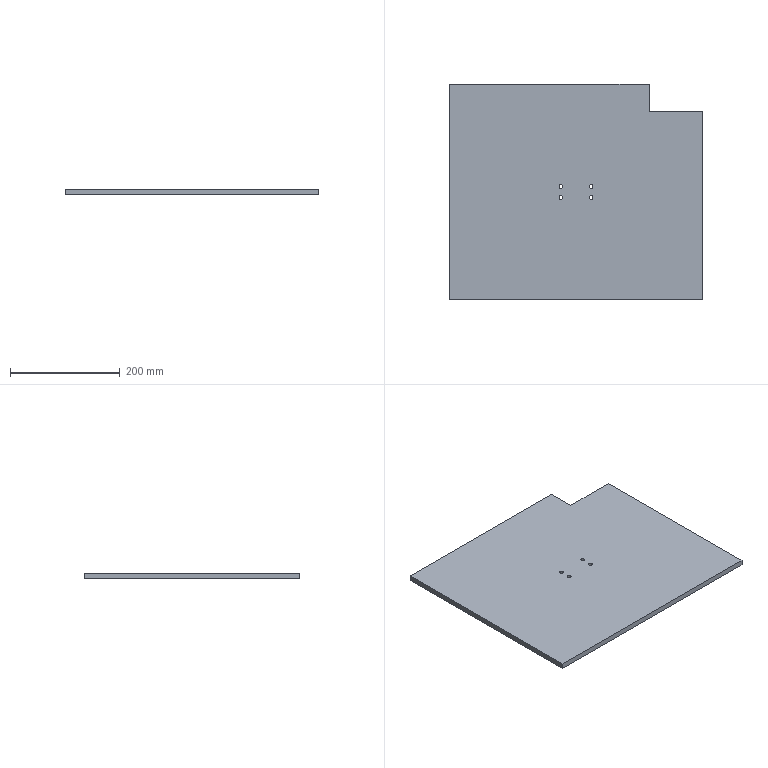Part | STEP file | Flat belt conveyor base plate | 1 solid | 16 faces | box 463 x 393.9 x 10 mm | volume 1773598 mm3 | cylinder 8 | plane 8 | commonest cylinder face diameters 6.8 x8
STEP:
#1=CARTESIAN_POINT('',(30.9,-38.75,10.));
#2=VERTEX_POINT('',#1);
#3=CARTESIAN_POINT('',(24.1,-38.75,10.));
#4=VERTEX_POINT('',#3);
#5=CARTESIAN_POINT('',(27.5,-38.75,10.));
#6=DIRECTION('',(0.,0.,-1.));
#7=DIRECTION('',(-1.,0.,0.));
#8=AXIS2_PLACEMENT_3D('',#5,#6,#7);
#9=CIRCLE('',#8,3.4);
#10=EDGE_CURVE('',#2,#4,#9,.T.);
#11=ORIENTED_EDGE('',*,*,#10,.F.);
#12=CARTESIAN_POINT('',(30.9,-38.75,0.));
#13=VERTEX_POINT('',#12);
#14=CARTESIAN_POINT('',(30.9,-38.75,0.));
#15=DIRECTION('',(0.,0.,-1.));
#16=VECTOR('',#15,1000.);
#17=LINE('',#14,#16);
#18=EDGE_CURVE('',#2,#13,#17,.T.);
#19=ORIENTED_EDGE('',*,*,#18,.T.);
#20=CARTESIAN_POINT('',(24.1,-38.75,0.));
#21=VERTEX_POINT('',#20);
#22=CARTESIAN_POINT('',(27.5,-38.75,0.));
#23=DIRECTION('',(0.,0.,-1.));
#24=DIRECTION('',(-1.,0.,0.));
#25=AXIS2_PLACEMENT_3D('',#22,#23,#24);
#26=CIRCLE('',#25,3.4);
#27=EDGE_CURVE('',#13,#21,#26,.T.);
#28=ORIENTED_EDGE('',*,*,#27,.T.);
#29=CARTESIAN_POINT('',(24.1,-38.75,0.));
#30=DIRECTION('',(0.,0.,-1.));
#31=VECTOR('',#30,1000.);
#32=LINE('',#29,#31);
#33=EDGE_CURVE('',#4,#21,#32,.T.);
#34=ORIENTED_EDGE('',*,*,#33,.F.);
#35=EDGE_LOOP('',(#11,#19,#28,#34));
#36=FACE_OUTER_BOUND('',#35,.T.);
#37=CARTESIAN_POINT('',(27.5,-38.75,0.));
#38=DIRECTION('',(0.,0.,-1.));
#39=DIRECTION('',(-1.,0.,0.));
#40=AXIS2_PLACEMENT_3D('',#37,#38,#39);
#41=CYLINDRICAL_SURFACE('',#40,3.4);
#42=ADVANCED_FACE('',(#36),#41,.F.);
#43=CARTESIAN_POINT('',(-24.1,-38.75,10.));
#44=VERTEX_POINT('',#43);
#45=CARTESIAN_POINT('',(-30.9,-38.75,10.));
#46=VERTEX_POINT('',#45);
#47=CARTESIAN_POINT('',(-27.5,-38.75,10.));
#48=DIRECTION('',(0.,0.,-1.));
#49=DIRECTION('',(-1.,0.,0.));
#50=AXIS2_PLACEMENT_3D('',#47,#48,#49);
#51=CIRCLE('',#50,3.4);
#52=EDGE_CURVE('',#44,#46,#51,.T.);
#53=ORIENTED_EDGE('',*,*,#52,.F.);
#54=CARTESIAN_POINT('',(-24.1,-38.75,0.));
#55=VERTEX_POINT('',#54);
#56=CARTESIAN_POINT('',(-24.1,-38.75,0.));
#57=DIRECTION('',(0.,0.,-1.));
#58=VECTOR('',#57,1000.);
#59=LINE('',#56,#58);
#60=EDGE_CURVE('',#44,#55,#59,.T.);
#61=ORIENTED_EDGE('',*,*,#60,.T.);
#62=CARTESIAN_POINT('',(-30.9,-38.75,0.));
#63=VERTEX_POINT('',#62);
#64=CARTESIAN_POINT('',(-27.5,-38.75,0.));
#65=DIRECTION('',(0.,0.,-1.));
#66=DIRECTION('',(-1.,0.,0.));
#67=AXIS2_PLACEMENT_3D('',#64,#65,#66);
#68=CIRCLE('',#67,3.4);
#69=EDGE_CURVE('',#55,#63,#68,.T.);
#70=ORIENTED_EDGE('',*,*,#69,.T.);
#71=CARTESIAN_POINT('',(-30.9,-38.75,0.));
#72=DIRECTION('',(0.,0.,-1.));
#73=VECTOR('',#72,1000.);
#74=LINE('',#71,#73);
#75=EDGE_CURVE('',#46,#63,#74,.T.);
#76=ORIENTED_EDGE('',*,*,#75,.F.);
#77=EDGE_LOOP('',(#53,#61,#70,#76));
#78=FACE_OUTER_BOUND('',#77,.T.);
#79=CARTESIAN_POINT('',(-27.5,-38.75,0.));
#80=DIRECTION('',(0.,0.,-1.));
#81=DIRECTION('',(-1.,0.,0.));
#82=AXIS2_PLACEMENT_3D('',#79,#80,#81);
#83=CYLINDRICAL_SURFACE('',#82,3.4);
#84=ADVANCED_FACE('',(#78),#83,.F.);
#85=CARTESIAN_POINT('',(-24.1,-18.75,10.));
#86=VERTEX_POINT('',#85);
#87=CARTESIAN_POINT('',(-30.9,-18.75,10.));
#88=VERTEX_POINT('',#87);
#89=CARTESIAN_POINT('',(-27.5,-18.75,10.));
#90=DIRECTION('',(0.,0.,-1.));
#91=DIRECTION('',(-1.,0.,0.));
#92=AXIS2_PLACEMENT_3D('',#89,#90,#91);
#93=CIRCLE('',#92,3.4);
#94=EDGE_CURVE('',#86,#88,#93,.T.);
#95=ORIENTED_EDGE('',*,*,#94,.F.);
#96=CARTESIAN_POINT('',(-24.1,-18.75,0.));
#97=VERTEX_POINT('',#96);
#98=CARTESIAN_POINT('',(-24.1,-18.75,0.));
#99=DIRECTION('',(0.,0.,-1.));
#100=VECTOR('',#99,1000.);
#101=LINE('',#98,#100);
#102=EDGE_CURVE('',#86,#97,#101,.T.);
#103=ORIENTED_EDGE('',*,*,#102,.T.);
#104=CARTESIAN_POINT('',(-30.9,-18.75,0.));
#105=VERTEX_POINT('',#104);
#106=CARTESIAN_POINT('',(-27.5,-18.75,0.));
#107=DIRECTION('',(0.,0.,-1.));
#108=DIRECTION('',(-1.,0.,0.));
#109=AXIS2_PLACEMENT_3D('',#106,#107,#108);
#110=CIRCLE('',#109,3.4);
#111=EDGE_CURVE('',#97,#105,#110,.T.);
#112=ORIENTED_EDGE('',*,*,#111,.T.);
#113=CARTESIAN_POINT('',(-30.9,-18.75,0.));
#114=DIRECTION('',(0.,0.,-1.));
#115=VECTOR('',#114,1000.);
#116=LINE('',#113,#115);
#117=EDGE_CURVE('',#88,#105,#116,.T.);
#118=ORIENTED_EDGE('',*,*,#117,.F.);
#119=EDGE_LOOP('',(#95,#103,#112,#118));
#120=FACE_OUTER_BOUND('',#119,.T.);
#121=CARTESIAN_POINT('',(-27.5,-18.75,0.));
#122=DIRECTION('',(0.,0.,-1.));
#123=DIRECTION('',(-1.,0.,0.));
#124=AXIS2_PLACEMENT_3D('',#121,#122,#123);
#125=CYLINDRICAL_SURFACE('',#124,3.4);
#126=ADVANCED_FACE('',(#120),#125,.F.);
#127=CARTESIAN_POINT('',(30.9,-18.75,10.));
#128=VERTEX_POINT('',#127);
#129=CARTESIAN_POINT('',(24.1,-18.75,10.));
#130=VERTEX_POINT('',#129);
#131=CARTESIAN_POINT('',(27.5,-18.75,10.));
#132=DIRECTION('',(0.,0.,-1.));
#133=DIRECTION('',(-1.,0.,0.));
#134=AXIS2_PLACEMENT_3D('',#131,#132,#133);
#135=CIRCLE('',#134,3.4);
#136=EDGE_CURVE('',#128,#130,#135,.T.);
#137=ORIENTED_EDGE('',*,*,#136,.F.);
#138=CARTESIAN_POINT('',(30.9,-18.75,0.));
#139=VERTEX_POINT('',#138);
#140=CARTESIAN_POINT('',(30.9,-18.75,0.));
#141=DIRECTION('',(0.,0.,-1.));
#142=VECTOR('',#141,1000.);
#143=LINE('',#140,#142);
#144=EDGE_CURVE('',#128,#139,#143,.T.);
#145=ORIENTED_EDGE('',*,*,#144,.T.);
#146=CARTESIAN_POINT('',(24.1,-18.75,0.));
#147=VERTEX_POINT('',#146);
#148=CARTESIAN_POINT('',(27.5,-18.75,0.));
#149=DIRECTION('',(0.,0.,-1.));
#150=DIRECTION('',(-1.,0.,0.));
#151=AXIS2_PLACEMENT_3D('',#148,#149,#150);
#152=CIRCLE('',#151,3.4);
#153=EDGE_CURVE('',#139,#147,#152,.T.);
#154=ORIENTED_EDGE('',*,*,#153,.T.);
#155=CARTESIAN_POINT('',(24.1,-18.75,0.));
#156=DIRECTION('',(0.,0.,-1.));
#157=VECTOR('',#156,1000.);
#158=LINE('',#155,#157);
#159=EDGE_CURVE('',#130,#147,#158,.T.);
#160=ORIENTED_EDGE('',*,*,#159,.F.);
#161=EDGE_LOOP('',(#137,#145,#154,#160));
#162=FACE_OUTER_BOUND('',#161,.T.);
#163=CARTESIAN_POINT('',(27.5,-18.75,0.));
#164=DIRECTION('',(0.,0.,-1.));
#165=DIRECTION('',(-1.,0.,0.));
#166=AXIS2_PLACEMENT_3D('',#163,#164,#165);
#167=CYLINDRICAL_SURFACE('',#166,3.4);
#168=ADVANCED_FACE('',(#162),#167,.F.);
#169=CARTESIAN_POINT('',(231.5,-225.7,0.));
#170=VERTEX_POINT('',#169);
#171=CARTESIAN_POINT('',(231.5,118.5,0.));
#172=VERTEX_POINT('',#171);
#173=CARTESIAN_POINT('',(231.5,-168.2,0.));
#174=DIRECTION('',(0.,1.,0.));
#175=VECTOR('',#174,1000.);
#176=LINE('',#173,#175);
#177=EDGE_CURVE('',#170,#172,#176,.T.);
#178=ORIENTED_EDGE('',*,*,#177,.T.);
#179=CARTESIAN_POINT('',(231.5,118.5,10.));
#180=VERTEX_POINT('',#179);
#181=CARTESIAN_POINT('',(231.5,118.5,0.));
#182=DIRECTION('',(0.,0.,1.));
#183=VECTOR('',#182,1000.);
#184=LINE('',#181,#183);
#185=EDGE_CURVE('',#172,#180,#184,.T.);
#186=ORIENTED_EDGE('',*,*,#185,.T.);
#187=CARTESIAN_POINT('',(231.5,-225.7,10.));
#188=VERTEX_POINT('',#187);
#189=CARTESIAN_POINT('',(231.5,-168.2,10.));
#190=DIRECTION('',(0.,1.,0.));
#191=VECTOR('',#190,1000.);
#192=LINE('',#189,#191);
#193=EDGE_CURVE('',#188,#180,#192,.T.);
#194=ORIENTED_EDGE('',*,*,#193,.F.);
#195=CARTESIAN_POINT('',(231.5,-225.7,-466.557));
#196=DIRECTION('',(0.,0.,1.));
#197=VECTOR('',#196,1000.);
#198=LINE('',#195,#197);
#199=EDGE_CURVE('',#170,#188,#198,.T.);
#200=ORIENTED_EDGE('',*,*,#199,.F.);
#201=EDGE_LOOP('',(#178,#186,#194,#200));
#202=FACE_OUTER_BOUND('',#201,.T.);
#203=CARTESIAN_POINT('',(231.5,-168.2,10.));
#204=DIRECTION('',(-1.,0.,0.));
#205=DIRECTION('',(0.,0.,1.));
#206=AXIS2_PLACEMENT_3D('',#203,#204,#205);
#207=PLANE('',#206);
#208=ADVANCED_FACE('',(#202),#207,.F.);
#209=CARTESIAN_POINT('',(133.5,168.2,10.));
#210=VERTEX_POINT('',#209);
#211=CARTESIAN_POINT('',(-231.5,168.2,10.));
#212=VERTEX_POINT('',#211);
#213=CARTESIAN_POINT('',(-231.5,168.2,10.));
#214=DIRECTION('',(-1.,0.,0.));
#215=VECTOR('',#214,1000.);
#216=LINE('',#213,#215);
#217=EDGE_CURVE('',#210,#212,#216,.T.);
#218=ORIENTED_EDGE('',*,*,#217,.F.);
#219=CARTESIAN_POINT('',(133.5,168.2,0.));
#220=VERTEX_POINT('',#219);
#221=CARTESIAN_POINT('',(133.5,168.2,0.));
#222=DIRECTION('',(0.,0.,1.));
#223=VECTOR('',#222,1000.);
#224=LINE('',#221,#223);
#225=EDGE_CURVE('',#220,#210,#224,.T.);
#226=ORIENTED_EDGE('',*,*,#225,.F.);
#227=CARTESIAN_POINT('',(-231.5,168.2,0.));
#228=VERTEX_POINT('',#227);
#229=CARTESIAN_POINT('',(-231.5,168.2,0.));
#230=DIRECTION('',(-1.,0.,0.));
#231=VECTOR('',#230,1000.);
#232=LINE('',#229,#231);
#233=EDGE_CURVE('',#220,#228,#232,.T.);
#234=ORIENTED_EDGE('',*,*,#233,.T.);
#235=CARTESIAN_POINT('',(-231.5,168.2,10.));
#236=DIRECTION('',(0.,0.,-1.));
#237=VECTOR('',#236,1000.);
#238=LINE('',#235,#237);
#239=EDGE_CURVE('',#212,#228,#238,.T.);
#240=ORIENTED_EDGE('',*,*,#239,.F.);
#241=EDGE_LOOP('',(#218,#226,#234,#240));
#242=FACE_OUTER_BOUND('',#241,.T.);
#243=CARTESIAN_POINT('',(-231.5,168.2,10.));
#244=DIRECTION('',(0.,-1.,0.));
#245=DIRECTION('',(0.,0.,-1.));
#246=AXIS2_PLACEMENT_3D('',#243,#244,#245);
#247=PLANE('',#246);
#248=ADVANCED_FACE('',(#242),#247,.F.);
#249=CARTESIAN_POINT('',(-231.5,-225.7,0.));
#250=VERTEX_POINT('',#249);
#251=CARTESIAN_POINT('',(-231.5,-168.2,0.));
#252=DIRECTION('',(0.,-1.,0.));
#253=VECTOR('',#252,1000.);
#254=LINE('',#251,#253);
#255=EDGE_CURVE('',#228,#250,#254,.T.);
#256=ORIENTED_EDGE('',*,*,#255,.T.);
#257=CARTESIAN_POINT('',(-231.5,-225.7,10.));
#258=VERTEX_POINT('',#257);
#259=CARTESIAN_POINT('',(-231.5,-225.7,-466.557));
#260=DIRECTION('',(0.,0.,1.));
#261=VECTOR('',#260,1000.);
#262=LINE('',#259,#261);
#263=EDGE_CURVE('',#250,#258,#262,.T.);
#264=ORIENTED_EDGE('',*,*,#263,.T.);
#265=CARTESIAN_POINT('',(-231.5,-168.2,10.));
#266=DIRECTION('',(0.,-1.,0.));
#267=VECTOR('',#266,1000.);
#268=LINE('',#265,#267);
#269=EDGE_CURVE('',#212,#258,#268,.T.);
#270=ORIENTED_EDGE('',*,*,#269,.F.);
#271=ORIENTED_EDGE('',*,*,#239,.T.);
#272=EDGE_LOOP('',(#256,#264,#270,#271));
#273=FACE_OUTER_BOUND('',#272,.T.);
#274=CARTESIAN_POINT('',(-231.5,-168.2,10.));
#275=DIRECTION('',(1.,0.,0.));
#276=DIRECTION('',(0.,0.,-1.));
#277=AXIS2_PLACEMENT_3D('',#274,#275,#276);
#278=PLANE('',#277);
#279=ADVANCED_FACE('',(#273),#278,.F.);
#280=CARTESIAN_POINT('',(27.5,-38.75,10.));
#281=DIRECTION('',(0.,0.,-1.));
#282=DIRECTION('',(-1.,0.,0.));
#283=AXIS2_PLACEMENT_3D('',#280,#281,#282);
#284=CIRCLE('',#283,3.4);
#285=EDGE_CURVE('',#4,#2,#284,.T.);
#286=ORIENTED_EDGE('',*,*,#285,.T.);
#287=ORIENTED_EDGE('',*,*,#10,.T.);
#288=EDGE_LOOP('',(#286,#287));
#289=FACE_BOUND('',#288,.T.);
#290=CARTESIAN_POINT('',(-27.5,-38.75,10.));
#291=DIRECTION('',(0.,0.,-1.));
#292=DIRECTION('',(-1.,0.,0.));
#293=AXIS2_PLACEMENT_3D('',#290,#291,#292);
#294=CIRCLE('',#293,3.4);
#295=EDGE_CURVE('',#46,#44,#294,.T.);
#296=ORIENTED_EDGE('',*,*,#295,.T.);
#297=ORIENTED_EDGE('',*,*,#52,.T.);
#298=EDGE_LOOP('',(#296,#297));
#299=FACE_BOUND('',#298,.T.);
#300=CARTESIAN_POINT('',(-27.5,-18.75,10.));
#301=DIRECTION('',(0.,0.,-1.));
#302=DIRECTION('',(-1.,0.,0.));
#303=AXIS2_PLACEMENT_3D('',#300,#301,#302);
#304=CIRCLE('',#303,3.4);
#305=EDGE_CURVE('',#88,#86,#304,.T.);
#306=ORIENTED_EDGE('',*,*,#305,.T.);
#307=ORIENTED_EDGE('',*,*,#94,.T.);
#308=EDGE_LOOP('',(#306,#307));
#309=FACE_BOUND('',#308,.T.);
#310=CARTESIAN_POINT('',(27.5,-18.75,10.));
#311=DIRECTION('',(0.,0.,-1.));
#312=DIRECTION('',(-1.,0.,0.));
#313=AXIS2_PLACEMENT_3D('',#310,#311,#312);
#314=CIRCLE('',#313,3.4);
#315=EDGE_CURVE('',#130,#128,#314,.T.);
#316=ORIENTED_EDGE('',*,*,#315,.T.);
#317=ORIENTED_EDGE('',*,*,#136,.T.);
#318=EDGE_LOOP('',(#316,#317));
#319=FACE_BOUND('',#318,.T.);
#320=CARTESIAN_POINT('',(133.5,118.5,10.));
#321=VERTEX_POINT('',#320);
#322=CARTESIAN_POINT('',(133.5,118.5,10.));
#323=DIRECTION('',(1.,0.,0.));
#324=VECTOR('',#323,1000.);
#325=LINE('',#322,#324);
#326=EDGE_CURVE('',#321,#180,#325,.T.);
#327=ORIENTED_EDGE('',*,*,#326,.F.);
#328=CARTESIAN_POINT('',(133.5,118.5,10.));
#329=DIRECTION('',(0.,-1.,0.));
#330=VECTOR('',#329,1000.);
#331=LINE('',#328,#330);
#332=EDGE_CURVE('',#210,#321,#331,.T.);
#333=ORIENTED_EDGE('',*,*,#332,.F.);
#334=ORIENTED_EDGE('',*,*,#217,.T.);
#335=ORIENTED_EDGE('',*,*,#269,.T.);
#336=CARTESIAN_POINT('',(-231.5,-225.7,10.));
#337=DIRECTION('',(1.,0.,0.));
#338=VECTOR('',#337,1000.);
#339=LINE('',#336,#338);
#340=EDGE_CURVE('',#258,#188,#339,.T.);
#341=ORIENTED_EDGE('',*,*,#340,.T.);
#342=ORIENTED_EDGE('',*,*,#193,.T.);
#343=EDGE_LOOP('',(#327,#333,#334,#335,#341,#342));
#344=FACE_OUTER_BOUND('',#343,.T.);
#345=CARTESIAN_POINT('',(0.,0.,10.));
#346=DIRECTION('',(0.,0.,-1.));
#347=DIRECTION('',(-1.,0.,0.));
#348=AXIS2_PLACEMENT_3D('',#345,#346,#347);
#349=PLANE('',#348);
#350=ADVANCED_FACE('',(#289,#299,#309,#319,#344),#349,.F.);
#351=CARTESIAN_POINT('',(27.5,-38.75,0.));
#352=DIRECTION('',(0.,0.,-1.));
#353=DIRECTION('',(-1.,0.,0.));
#354=AXIS2_PLACEMENT_3D('',#351,#352,#353);
#355=CIRCLE('',#354,3.4);
#356=EDGE_CURVE('',#21,#13,#355,.T.);
#357=ORIENTED_EDGE('',*,*,#356,.F.);
#358=ORIENTED_EDGE('',*,*,#27,.F.);
#359=EDGE_LOOP('',(#357,#358));
#360=FACE_BOUND('',#359,.T.);
#361=CARTESIAN_POINT('',(-27.5,-38.75,0.));
#362=DIRECTION('',(0.,0.,-1.));
#363=DIRECTION('',(-1.,0.,0.));
#364=AXIS2_PLACEMENT_3D('',#361,#362,#363);
#365=CIRCLE('',#364,3.4);
#366=EDGE_CURVE('',#63,#55,#365,.T.);
#367=ORIENTED_EDGE('',*,*,#366,.F.);
#368=ORIENTED_EDGE('',*,*,#69,.F.);
#369=EDGE_LOOP('',(#367,#368));
#370=FACE_BOUND('',#369,.T.);
#371=CARTESIAN_POINT('',(-27.5,-18.75,0.));
#372=DIRECTION('',(0.,0.,-1.));
#373=DIRECTION('',(-1.,0.,0.));
#374=AXIS2_PLACEMENT_3D('',#371,#372,#373);
#375=CIRCLE('',#374,3.4);
#376=EDGE_CURVE('',#105,#97,#375,.T.);
#377=ORIENTED_EDGE('',*,*,#376,.F.);
#378=ORIENTED_EDGE('',*,*,#111,.F.);
#379=EDGE_LOOP('',(#377,#378));
#380=FACE_BOUND('',#379,.T.);
#381=CARTESIAN_POINT('',(27.5,-18.75,0.));
#382=DIRECTION('',(0.,0.,-1.));
#383=DIRECTION('',(-1.,0.,0.));
#384=AXIS2_PLACEMENT_3D('',#381,#382,#383);
#385=CIRCLE('',#384,3.4);
#386=EDGE_CURVE('',#147,#139,#385,.T.);
#387=ORIENTED_EDGE('',*,*,#386,.F.);
#388=ORIENTED_EDGE('',*,*,#153,.F.);
#389=EDGE_LOOP('',(#387,#388));
#390=FACE_BOUND('',#389,.T.);
#391=CARTESIAN_POINT('',(133.5,118.5,0.));
#392=VERTEX_POINT('',#391);
#393=CARTESIAN_POINT('',(133.5,118.5,0.));
#394=DIRECTION('',(0.,-1.,0.));
#395=VECTOR('',#394,1000.);
#396=LINE('',#393,#395);
#397=EDGE_CURVE('',#220,#392,#396,.T.);
#398=ORIENTED_EDGE('',*,*,#397,.T.);
#399=CARTESIAN_POINT('',(133.5,118.5,0.));
#400=DIRECTION('',(1.,0.,0.));
#401=VECTOR('',#400,1000.);
#402=LINE('',#399,#401);
#403=EDGE_CURVE('',#392,#172,#402,.T.);
#404=ORIENTED_EDGE('',*,*,#403,.T.);
#405=ORIENTED_EDGE('',*,*,#177,.F.);
#406=CARTESIAN_POINT('',(-231.5,-225.7,0.));
#407=DIRECTION('',(1.,0.,0.));
#408=VECTOR('',#407,1000.);
#409=LINE('',#406,#408);
#410=EDGE_CURVE('',#250,#170,#409,.T.);
#411=ORIENTED_EDGE('',*,*,#410,.F.);
#412=ORIENTED_EDGE('',*,*,#255,.F.);
#413=ORIENTED_EDGE('',*,*,#233,.F.);
#414=EDGE_LOOP('',(#398,#404,#405,#411,#412,#413));
#415=FACE_OUTER_BOUND('',#414,.T.);
#416=CARTESIAN_POINT('',(0.,0.,0.));
#417=DIRECTION('',(0.,0.,-1.));
#418=DIRECTION('',(-1.,0.,0.));
#419=AXIS2_PLACEMENT_3D('',#416,#417,#418);
#420=PLANE('',#419);
#421=ADVANCED_FACE('',(#360,#370,#380,#390,#415),#420,.T.);
#422=ORIENTED_EDGE('',*,*,#332,.T.);
#423=CARTESIAN_POINT('',(133.5,118.5,0.));
#424=DIRECTION('',(0.,0.,1.));
#425=VECTOR('',#424,1000.);
#426=LINE('',#423,#425);
#427=EDGE_CURVE('',#392,#321,#426,.T.);
#428=ORIENTED_EDGE('',*,*,#427,.F.);
#429=ORIENTED_EDGE('',*,*,#397,.F.);
#430=ORIENTED_EDGE('',*,*,#225,.T.);
#431=EDGE_LOOP('',(#422,#428,#429,#430));
#432=FACE_OUTER_BOUND('',#431,.T.);
#433=CARTESIAN_POINT('',(133.5,118.5,0.));
#434=DIRECTION('',(-1.,0.,0.));
#435=DIRECTION('',(0.,0.,1.));
#436=AXIS2_PLACEMENT_3D('',#433,#434,#435);
#437=PLANE('',#436);
#438=ADVANCED_FACE('',(#432),#437,.F.);
#439=ORIENTED_EDGE('',*,*,#326,.T.);
#440=ORIENTED_EDGE('',*,*,#185,.F.);
#441=ORIENTED_EDGE('',*,*,#403,.F.);
#442=ORIENTED_EDGE('',*,*,#427,.T.);
#443=EDGE_LOOP('',(#439,#440,#441,#442));
#444=FACE_OUTER_BOUND('',#443,.T.);
#445=CARTESIAN_POINT('',(133.5,118.5,0.));
#446=DIRECTION('',(0.,-1.,0.));
#447=DIRECTION('',(0.,0.,-1.));
#448=AXIS2_PLACEMENT_3D('',#445,#446,#447);
#449=PLANE('',#448);
#450=ADVANCED_FACE('',(#444),#449,.F.);
#451=ORIENTED_EDGE('',*,*,#263,.F.);
#452=ORIENTED_EDGE('',*,*,#410,.T.);
#453=ORIENTED_EDGE('',*,*,#199,.T.);
#454=ORIENTED_EDGE('',*,*,#340,.F.);
#455=EDGE_LOOP('',(#451,#452,#453,#454));
#456=FACE_OUTER_BOUND('',#455,.T.);
#457=CARTESIAN_POINT('',(-231.5,-225.7,-466.557));
#458=DIRECTION('',(0.,-1.,0.));
#459=DIRECTION('',(0.,0.,-1.));
#460=AXIS2_PLACEMENT_3D('',#457,#458,#459);
#461=PLANE('',#460);
#462=ADVANCED_FACE('',(#456),#461,.T.);
#463=ORIENTED_EDGE('',*,*,#144,.F.);
#464=ORIENTED_EDGE('',*,*,#315,.F.);
#465=ORIENTED_EDGE('',*,*,#159,.T.);
#466=ORIENTED_EDGE('',*,*,#386,.T.);
#467=EDGE_LOOP('',(#463,#464,#465,#466));
#468=FACE_OUTER_BOUND('',#467,.T.);
#469=CARTESIAN_POINT('',(27.5,-18.75,0.));
#470=DIRECTION('',(0.,0.,-1.));
#471=DIRECTION('',(-1.,0.,0.));
#472=AXIS2_PLACEMENT_3D('',#469,#470,#471);
#473=CYLINDRICAL_SURFACE('',#472,3.4);
#474=ADVANCED_FACE('',(#468),#473,.F.);
#475=ORIENTED_EDGE('',*,*,#102,.F.);
#476=ORIENTED_EDGE('',*,*,#305,.F.);
#477=ORIENTED_EDGE('',*,*,#117,.T.);
#478=ORIENTED_EDGE('',*,*,#376,.T.);
#479=EDGE_LOOP('',(#475,#476,#477,#478));
#480=FACE_OUTER_BOUND('',#479,.T.);
#481=CARTESIAN_POINT('',(-27.5,-18.75,0.));
#482=DIRECTION('',(0.,0.,-1.));
#483=DIRECTION('',(-1.,0.,0.));
#484=AXIS2_PLACEMENT_3D('',#481,#482,#483);
#485=CYLINDRICAL_SURFACE('',#484,3.4);
#486=ADVANCED_FACE('',(#480),#485,.F.);
#487=ORIENTED_EDGE('',*,*,#60,.F.);
#488=ORIENTED_EDGE('',*,*,#295,.F.);
#489=ORIENTED_EDGE('',*,*,#75,.T.);
#490=ORIENTED_EDGE('',*,*,#366,.T.);
#491=EDGE_LOOP('',(#487,#488,#489,#490));
#492=FACE_OUTER_BOUND('',#491,.T.);
#493=CARTESIAN_POINT('',(-27.5,-38.75,0.));
#494=DIRECTION('',(0.,0.,-1.));
#495=DIRECTION('',(-1.,0.,0.));
#496=AXIS2_PLACEMENT_3D('',#493,#494,#495);
#497=CYLINDRICAL_SURFACE('',#496,3.4);
#498=ADVANCED_FACE('',(#492),#497,.F.);
#499=ORIENTED_EDGE('',*,*,#18,.F.);
#500=ORIENTED_EDGE('',*,*,#285,.F.);
#501=ORIENTED_EDGE('',*,*,#33,.T.);
#502=ORIENTED_EDGE('',*,*,#356,.T.);
#503=EDGE_LOOP('',(#499,#500,#501,#502));
#504=FACE_OUTER_BOUND('',#503,.T.);
#505=CARTESIAN_POINT('',(27.5,-38.75,0.));
#506=DIRECTION('',(0.,0.,-1.));
#507=DIRECTION('',(-1.,0.,0.));
#508=AXIS2_PLACEMENT_3D('',#505,#506,#507);
#509=CYLINDRICAL_SURFACE('',#508,3.4);
#510=ADVANCED_FACE('',(#504),#509,.F.);
#511=CLOSED_SHELL('',(#42,#84,#126,#168,#208,#248,#279,#350,#421,#438,#450,#462,#474,#486,#498,#510));
#512=MANIFOLD_SOLID_BREP('',#511);
#513=CARTESIAN_POINT('',(0.,0.,0.));
#514=DIRECTION('',(0.,0.,1.));
#515=DIRECTION('',(1.,0.,0.));
#516=AXIS2_PLACEMENT_3D('',#513,#514,#515);
#517=(LENGTH_UNIT()NAMED_UNIT(*)SI_UNIT(.MILLI.,.METRE.));
#518=UNCERTAINTY_MEASURE_WITH_UNIT(LENGTH_MEASURE(0.00001),#517,'','');
#519=(NAMED_UNIT(*)PLANE_ANGLE_UNIT()SI_UNIT($,.RADIAN.));
#520=(NAMED_UNIT(*)SI_UNIT($,.STERADIAN.)SOLID_ANGLE_UNIT());
#521=(GEOMETRIC_REPRESENTATION_CONTEXT(3)GLOBAL_UNCERTAINTY_ASSIGNED_CONTEXT((#518))GLOBAL_UNIT_ASSIGNED_CONTEXT((#517,#519,#520))REPRESENTATION_CONTEXT('',''));
#522=ADVANCED_BREP_SHAPE_REPRESENTATION('',(#512,#516),#521);